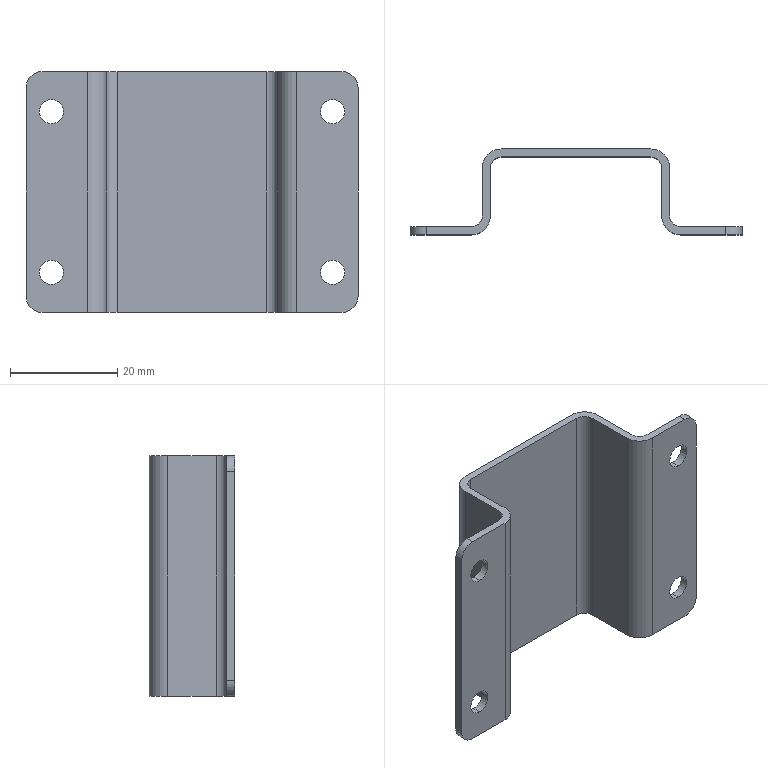Part | SolidWorks | features BaseBody 1 | 1 solid | 34 faces | box 62 x 16 x 45 mm | volume 5717 mm3 | cylinder 20 | plane 14 | commonest cylinder face diameters 4.5 x8 4 x4 6 x4 7 x4
STEP:
#1=CARTESIAN_POINT('',(-26.25,-16.,-17.25));
#2=VERTEX_POINT('',#1);
#3=CARTESIAN_POINT('',(-26.25,-16.,-12.75));
#4=VERTEX_POINT('',#3);
#5=CARTESIAN_POINT('',(-26.25,-16.,-15.));
#6=DIRECTION('',(0.,1.,0.));
#7=DIRECTION('',(0.,0.,1.));
#8=AXIS2_PLACEMENT_3D('',#5,#6,#7);
#9=CIRCLE('',#8,2.25);
#10=EDGE_CURVE('',#2,#4,#9,.T.);
#11=ORIENTED_EDGE('',*,*,#10,.F.);
#12=CARTESIAN_POINT('',(-26.25,-14.5,-17.25));
#13=VERTEX_POINT('',#12);
#14=CARTESIAN_POINT('',(-26.25,-14.5,-17.25));
#15=DIRECTION('',(0.,1.,0.));
#16=VECTOR('',#15,1000.);
#17=LINE('',#14,#16);
#18=EDGE_CURVE('',#2,#13,#17,.T.);
#19=ORIENTED_EDGE('',*,*,#18,.T.);
#20=CARTESIAN_POINT('',(-26.25,-14.5,-12.75));
#21=VERTEX_POINT('',#20);
#22=CARTESIAN_POINT('',(-26.25,-14.5,-15.));
#23=DIRECTION('',(0.,1.,0.));
#24=DIRECTION('',(0.,0.,1.));
#25=AXIS2_PLACEMENT_3D('',#22,#23,#24);
#26=CIRCLE('',#25,2.25);
#27=EDGE_CURVE('',#13,#21,#26,.T.);
#28=ORIENTED_EDGE('',*,*,#27,.T.);
#29=CARTESIAN_POINT('',(-26.25,-14.5,-12.75));
#30=DIRECTION('',(0.,1.,0.));
#31=VECTOR('',#30,1000.);
#32=LINE('',#29,#31);
#33=EDGE_CURVE('',#4,#21,#32,.T.);
#34=ORIENTED_EDGE('',*,*,#33,.F.);
#35=EDGE_LOOP('',(#11,#19,#28,#34));
#36=FACE_OUTER_BOUND('',#35,.T.);
#37=CARTESIAN_POINT('',(-26.25,-14.5,-15.));
#38=DIRECTION('',(0.,1.,0.));
#39=DIRECTION('',(0.,0.,1.));
#40=AXIS2_PLACEMENT_3D('',#37,#38,#39);
#41=CYLINDRICAL_SURFACE('',#40,2.25);
#42=ADVANCED_FACE('',(#36),#41,.F.);
#43=CARTESIAN_POINT('',(-26.25,-16.,12.75));
#44=VERTEX_POINT('',#43);
#45=CARTESIAN_POINT('',(-26.25,-16.,17.25));
#46=VERTEX_POINT('',#45);
#47=CARTESIAN_POINT('',(-26.25,-16.,15.));
#48=DIRECTION('',(0.,1.,0.));
#49=DIRECTION('',(0.,0.,1.));
#50=AXIS2_PLACEMENT_3D('',#47,#48,#49);
#51=CIRCLE('',#50,2.25);
#52=EDGE_CURVE('',#44,#46,#51,.T.);
#53=ORIENTED_EDGE('',*,*,#52,.F.);
#54=CARTESIAN_POINT('',(-26.25,-14.5,12.75));
#55=VERTEX_POINT('',#54);
#56=CARTESIAN_POINT('',(-26.25,-14.5,12.75));
#57=DIRECTION('',(0.,1.,0.));
#58=VECTOR('',#57,1000.);
#59=LINE('',#56,#58);
#60=EDGE_CURVE('',#44,#55,#59,.T.);
#61=ORIENTED_EDGE('',*,*,#60,.T.);
#62=CARTESIAN_POINT('',(-26.25,-14.5,17.25));
#63=VERTEX_POINT('',#62);
#64=CARTESIAN_POINT('',(-26.25,-14.5,15.));
#65=DIRECTION('',(0.,1.,0.));
#66=DIRECTION('',(0.,0.,1.));
#67=AXIS2_PLACEMENT_3D('',#64,#65,#66);
#68=CIRCLE('',#67,2.25);
#69=EDGE_CURVE('',#55,#63,#68,.T.);
#70=ORIENTED_EDGE('',*,*,#69,.T.);
#71=CARTESIAN_POINT('',(-26.25,-14.5,17.25));
#72=DIRECTION('',(0.,1.,0.));
#73=VECTOR('',#72,1000.);
#74=LINE('',#71,#73);
#75=EDGE_CURVE('',#46,#63,#74,.T.);
#76=ORIENTED_EDGE('',*,*,#75,.F.);
#77=EDGE_LOOP('',(#53,#61,#70,#76));
#78=FACE_OUTER_BOUND('',#77,.T.);
#79=CARTESIAN_POINT('',(-26.25,-14.5,15.));
#80=DIRECTION('',(0.,1.,0.));
#81=DIRECTION('',(0.,0.,1.));
#82=AXIS2_PLACEMENT_3D('',#79,#80,#81);
#83=CYLINDRICAL_SURFACE('',#82,2.25);
#84=ADVANCED_FACE('',(#78),#83,.F.);
#85=CARTESIAN_POINT('',(26.25,-16.,12.75));
#86=VERTEX_POINT('',#85);
#87=CARTESIAN_POINT('',(26.25,-16.,17.25));
#88=VERTEX_POINT('',#87);
#89=CARTESIAN_POINT('',(26.25,-16.,15.));
#90=DIRECTION('',(0.,1.,0.));
#91=DIRECTION('',(0.,0.,1.));
#92=AXIS2_PLACEMENT_3D('',#89,#90,#91);
#93=CIRCLE('',#92,2.25);
#94=EDGE_CURVE('',#86,#88,#93,.T.);
#95=ORIENTED_EDGE('',*,*,#94,.F.);
#96=CARTESIAN_POINT('',(26.25,-14.5,12.75));
#97=VERTEX_POINT('',#96);
#98=CARTESIAN_POINT('',(26.25,-14.5,12.75));
#99=DIRECTION('',(0.,1.,0.));
#100=VECTOR('',#99,1000.);
#101=LINE('',#98,#100);
#102=EDGE_CURVE('',#86,#97,#101,.T.);
#103=ORIENTED_EDGE('',*,*,#102,.T.);
#104=CARTESIAN_POINT('',(26.25,-14.5,17.25));
#105=VERTEX_POINT('',#104);
#106=CARTESIAN_POINT('',(26.25,-14.5,15.));
#107=DIRECTION('',(0.,1.,0.));
#108=DIRECTION('',(0.,0.,1.));
#109=AXIS2_PLACEMENT_3D('',#106,#107,#108);
#110=CIRCLE('',#109,2.25);
#111=EDGE_CURVE('',#97,#105,#110,.T.);
#112=ORIENTED_EDGE('',*,*,#111,.T.);
#113=CARTESIAN_POINT('',(26.25,-14.5,17.25));
#114=DIRECTION('',(0.,1.,0.));
#115=VECTOR('',#114,1000.);
#116=LINE('',#113,#115);
#117=EDGE_CURVE('',#88,#105,#116,.T.);
#118=ORIENTED_EDGE('',*,*,#117,.F.);
#119=EDGE_LOOP('',(#95,#103,#112,#118));
#120=FACE_OUTER_BOUND('',#119,.T.);
#121=CARTESIAN_POINT('',(26.25,-14.5,15.));
#122=DIRECTION('',(0.,1.,0.));
#123=DIRECTION('',(0.,0.,1.));
#124=AXIS2_PLACEMENT_3D('',#121,#122,#123);
#125=CYLINDRICAL_SURFACE('',#124,2.25);
#126=ADVANCED_FACE('',(#120),#125,.F.);
#127=CARTESIAN_POINT('',(26.25,-16.,-17.25));
#128=VERTEX_POINT('',#127);
#129=CARTESIAN_POINT('',(26.25,-16.,-12.75));
#130=VERTEX_POINT('',#129);
#131=CARTESIAN_POINT('',(26.25,-16.,-15.));
#132=DIRECTION('',(0.,1.,0.));
#133=DIRECTION('',(0.,0.,1.));
#134=AXIS2_PLACEMENT_3D('',#131,#132,#133);
#135=CIRCLE('',#134,2.25);
#136=EDGE_CURVE('',#128,#130,#135,.T.);
#137=ORIENTED_EDGE('',*,*,#136,.F.);
#138=CARTESIAN_POINT('',(26.25,-14.5,-17.25));
#139=VERTEX_POINT('',#138);
#140=CARTESIAN_POINT('',(26.25,-14.5,-17.25));
#141=DIRECTION('',(0.,1.,0.));
#142=VECTOR('',#141,1000.);
#143=LINE('',#140,#142);
#144=EDGE_CURVE('',#128,#139,#143,.T.);
#145=ORIENTED_EDGE('',*,*,#144,.T.);
#146=CARTESIAN_POINT('',(26.25,-14.5,-12.75));
#147=VERTEX_POINT('',#146);
#148=CARTESIAN_POINT('',(26.25,-14.5,-15.));
#149=DIRECTION('',(0.,1.,0.));
#150=DIRECTION('',(0.,0.,1.));
#151=AXIS2_PLACEMENT_3D('',#148,#149,#150);
#152=CIRCLE('',#151,2.25);
#153=EDGE_CURVE('',#139,#147,#152,.T.);
#154=ORIENTED_EDGE('',*,*,#153,.T.);
#155=CARTESIAN_POINT('',(26.25,-14.5,-12.75));
#156=DIRECTION('',(0.,1.,0.));
#157=VECTOR('',#156,1000.);
#158=LINE('',#155,#157);
#159=EDGE_CURVE('',#130,#147,#158,.T.);
#160=ORIENTED_EDGE('',*,*,#159,.F.);
#161=EDGE_LOOP('',(#137,#145,#154,#160));
#162=FACE_OUTER_BOUND('',#161,.T.);
#163=CARTESIAN_POINT('',(26.25,-14.5,-15.));
#164=DIRECTION('',(0.,1.,0.));
#165=DIRECTION('',(0.,0.,1.));
#166=AXIS2_PLACEMENT_3D('',#163,#164,#165);
#167=CYLINDRICAL_SURFACE('',#166,2.25);
#168=ADVANCED_FACE('',(#162),#167,.F.);
#169=CARTESIAN_POINT('',(28.,-16.,-22.5));
#170=VERTEX_POINT('',#169);
#171=CARTESIAN_POINT('',(31.,-16.,-19.5));
#172=VERTEX_POINT('',#171);
#173=CARTESIAN_POINT('',(28.,-16.,-19.5));
#174=DIRECTION('',(0.,-1.,0.));
#175=DIRECTION('',(0.,0.,1.));
#176=AXIS2_PLACEMENT_3D('',#173,#174,#175);
#177=CIRCLE('',#176,3.);
#178=EDGE_CURVE('',#170,#172,#177,.T.);
#179=ORIENTED_EDGE('',*,*,#178,.F.);
#180=CARTESIAN_POINT('',(28.,-14.5,-22.5));
#181=VERTEX_POINT('',#180);
#182=CARTESIAN_POINT('',(28.,-16.,-22.5));
#183=DIRECTION('',(0.,-1.,0.));
#184=VECTOR('',#183,1000.);
#185=LINE('',#182,#184);
#186=EDGE_CURVE('',#181,#170,#185,.T.);
#187=ORIENTED_EDGE('',*,*,#186,.F.);
#188=CARTESIAN_POINT('',(31.,-14.5,-19.5));
#189=VERTEX_POINT('',#188);
#190=CARTESIAN_POINT('',(28.,-14.5,-19.5));
#191=DIRECTION('',(0.,1.,0.));
#192=DIRECTION('',(0.,0.,1.));
#193=AXIS2_PLACEMENT_3D('',#190,#191,#192);
#194=CIRCLE('',#193,3.);
#195=EDGE_CURVE('',#189,#181,#194,.T.);
#196=ORIENTED_EDGE('',*,*,#195,.F.);
#197=CARTESIAN_POINT('',(31.,-16.,-19.5));
#198=DIRECTION('',(0.,1.,0.));
#199=VECTOR('',#198,1000.);
#200=LINE('',#197,#199);
#201=EDGE_CURVE('',#172,#189,#200,.T.);
#202=ORIENTED_EDGE('',*,*,#201,.F.);
#203=EDGE_LOOP('',(#179,#187,#196,#202));
#204=FACE_OUTER_BOUND('',#203,.T.);
#205=CARTESIAN_POINT('',(28.,-16.,-19.5));
#206=DIRECTION('',(0.,1.,0.));
#207=DIRECTION('',(-1.,0.,0.));
#208=AXIS2_PLACEMENT_3D('',#205,#206,#207);
#209=CYLINDRICAL_SURFACE('',#208,3.);
#210=ADVANCED_FACE('',(#204),#209,.T.);
#211=CARTESIAN_POINT('',(31.,-16.,19.5));
#212=VERTEX_POINT('',#211);
#213=CARTESIAN_POINT('',(28.,-16.,22.5));
#214=VERTEX_POINT('',#213);
#215=CARTESIAN_POINT('',(28.,-16.,19.5));
#216=DIRECTION('',(0.,-1.,0.));
#217=DIRECTION('',(0.,0.,1.));
#218=AXIS2_PLACEMENT_3D('',#215,#216,#217);
#219=CIRCLE('',#218,3.);
#220=EDGE_CURVE('',#212,#214,#219,.T.);
#221=ORIENTED_EDGE('',*,*,#220,.F.);
#222=CARTESIAN_POINT('',(31.,-14.5,19.5));
#223=VERTEX_POINT('',#222);
#224=CARTESIAN_POINT('',(31.,-16.,19.5));
#225=DIRECTION('',(0.,-1.,0.));
#226=VECTOR('',#225,1000.);
#227=LINE('',#224,#226);
#228=EDGE_CURVE('',#223,#212,#227,.T.);
#229=ORIENTED_EDGE('',*,*,#228,.F.);
#230=CARTESIAN_POINT('',(28.,-14.5,22.5));
#231=VERTEX_POINT('',#230);
#232=CARTESIAN_POINT('',(28.,-14.5,19.5));
#233=DIRECTION('',(0.,1.,0.));
#234=DIRECTION('',(0.,0.,1.));
#235=AXIS2_PLACEMENT_3D('',#232,#233,#234);
#236=CIRCLE('',#235,3.);
#237=EDGE_CURVE('',#231,#223,#236,.T.);
#238=ORIENTED_EDGE('',*,*,#237,.F.);
#239=CARTESIAN_POINT('',(28.,-16.,22.5));
#240=DIRECTION('',(0.,1.,0.));
#241=VECTOR('',#240,1000.);
#242=LINE('',#239,#241);
#243=EDGE_CURVE('',#214,#231,#242,.T.);
#244=ORIENTED_EDGE('',*,*,#243,.F.);
#245=EDGE_LOOP('',(#221,#229,#238,#244));
#246=FACE_OUTER_BOUND('',#245,.T.);
#247=CARTESIAN_POINT('',(28.,-16.,19.5));
#248=DIRECTION('',(0.,1.,0.));
#249=DIRECTION('',(-1.,0.,0.));
#250=AXIS2_PLACEMENT_3D('',#247,#248,#249);
#251=CYLINDRICAL_SURFACE('',#250,3.);
#252=ADVANCED_FACE('',(#246),#251,.T.);
#253=CARTESIAN_POINT('',(-28.,-16.,22.5));
#254=VERTEX_POINT('',#253);
#255=CARTESIAN_POINT('',(-31.,-16.,19.5));
#256=VERTEX_POINT('',#255);
#257=CARTESIAN_POINT('',(-28.,-16.,19.5));
#258=DIRECTION('',(0.,-1.,0.));
#259=DIRECTION('',(0.,0.,1.));
#260=AXIS2_PLACEMENT_3D('',#257,#258,#259);
#261=CIRCLE('',#260,3.);
#262=EDGE_CURVE('',#254,#256,#261,.T.);
#263=ORIENTED_EDGE('',*,*,#262,.F.);
#264=CARTESIAN_POINT('',(-28.,-14.5,22.5));
#265=VERTEX_POINT('',#264);
#266=CARTESIAN_POINT('',(-28.,-16.,22.5));
#267=DIRECTION('',(0.,-1.,0.));
#268=VECTOR('',#267,1000.);
#269=LINE('',#266,#268);
#270=EDGE_CURVE('',#265,#254,#269,.T.);
#271=ORIENTED_EDGE('',*,*,#270,.F.);
#272=CARTESIAN_POINT('',(-31.,-14.5,19.5));
#273=VERTEX_POINT('',#272);
#274=CARTESIAN_POINT('',(-28.,-14.5,19.5));
#275=DIRECTION('',(0.,1.,0.));
#276=DIRECTION('',(0.,0.,1.));
#277=AXIS2_PLACEMENT_3D('',#274,#275,#276);
#278=CIRCLE('',#277,3.);
#279=EDGE_CURVE('',#273,#265,#278,.T.);
#280=ORIENTED_EDGE('',*,*,#279,.F.);
#281=CARTESIAN_POINT('',(-31.,-16.,19.5));
#282=DIRECTION('',(0.,1.,0.));
#283=VECTOR('',#282,1000.);
#284=LINE('',#281,#283);
#285=EDGE_CURVE('',#256,#273,#284,.T.);
#286=ORIENTED_EDGE('',*,*,#285,.F.);
#287=EDGE_LOOP('',(#263,#271,#280,#286));
#288=FACE_OUTER_BOUND('',#287,.T.);
#289=CARTESIAN_POINT('',(-28.,-16.,19.5));
#290=DIRECTION('',(0.,1.,0.));
#291=DIRECTION('',(-1.,0.,0.));
#292=AXIS2_PLACEMENT_3D('',#289,#290,#291);
#293=CYLINDRICAL_SURFACE('',#292,3.);
#294=ADVANCED_FACE('',(#288),#293,.T.);
#295=CARTESIAN_POINT('',(-31.,-16.,-19.5));
#296=VERTEX_POINT('',#295);
#297=CARTESIAN_POINT('',(-28.,-16.,-22.5));
#298=VERTEX_POINT('',#297);
#299=CARTESIAN_POINT('',(-28.,-16.,-19.5));
#300=DIRECTION('',(0.,-1.,0.));
#301=DIRECTION('',(0.,0.,1.));
#302=AXIS2_PLACEMENT_3D('',#299,#300,#301);
#303=CIRCLE('',#302,3.);
#304=EDGE_CURVE('',#296,#298,#303,.T.);
#305=ORIENTED_EDGE('',*,*,#304,.F.);
#306=CARTESIAN_POINT('',(-31.,-14.5,-19.5));
#307=VERTEX_POINT('',#306);
#308=CARTESIAN_POINT('',(-31.,-16.,-19.5));
#309=DIRECTION('',(0.,-1.,0.));
#310=VECTOR('',#309,1000.);
#311=LINE('',#308,#310);
#312=EDGE_CURVE('',#307,#296,#311,.T.);
#313=ORIENTED_EDGE('',*,*,#312,.F.);
#314=CARTESIAN_POINT('',(-28.,-14.5,-22.5));
#315=VERTEX_POINT('',#314);
#316=CARTESIAN_POINT('',(-28.,-14.5,-19.5));
#317=DIRECTION('',(0.,1.,0.));
#318=DIRECTION('',(0.,0.,1.));
#319=AXIS2_PLACEMENT_3D('',#316,#317,#318);
#320=CIRCLE('',#319,3.);
#321=EDGE_CURVE('',#315,#307,#320,.T.);
#322=ORIENTED_EDGE('',*,*,#321,.F.);
#323=CARTESIAN_POINT('',(-28.,-16.,-22.5));
#324=DIRECTION('',(0.,1.,0.));
#325=VECTOR('',#324,1000.);
#326=LINE('',#323,#325);
#327=EDGE_CURVE('',#298,#315,#326,.T.);
#328=ORIENTED_EDGE('',*,*,#327,.F.);
#329=EDGE_LOOP('',(#305,#313,#322,#328));
#330=FACE_OUTER_BOUND('',#329,.T.);
#331=CARTESIAN_POINT('',(-28.,-16.,-19.5));
#332=DIRECTION('',(0.,1.,0.));
#333=DIRECTION('',(-1.,0.,0.));
#334=AXIS2_PLACEMENT_3D('',#331,#332,#333);
#335=CYLINDRICAL_SURFACE('',#334,3.);
#336=ADVANCED_FACE('',(#330),#335,.T.);
#337=CARTESIAN_POINT('',(31.,-14.5,22.5));
#338=DIRECTION('',(0.,0.,1.));
#339=VECTOR('',#338,1000.);
#340=LINE('',#337,#339);
#341=EDGE_CURVE('',#189,#223,#340,.T.);
#342=ORIENTED_EDGE('',*,*,#341,.T.);
#343=ORIENTED_EDGE('',*,*,#228,.T.);
#344=CARTESIAN_POINT('',(31.,-16.,0.));
#345=DIRECTION('',(0.,0.,1.));
#346=VECTOR('',#345,1000.);
#347=LINE('',#344,#346);
#348=EDGE_CURVE('',#172,#212,#347,.T.);
#349=ORIENTED_EDGE('',*,*,#348,.F.);
#350=ORIENTED_EDGE('',*,*,#201,.T.);
#351=EDGE_LOOP('',(#342,#343,#349,#350));
#352=FACE_OUTER_BOUND('',#351,.T.);
#353=CARTESIAN_POINT('',(31.,-16.,22.5));
#354=DIRECTION('',(-1.,0.,0.));
#355=DIRECTION('',(0.,1.,0.));
#356=AXIS2_PLACEMENT_3D('',#353,#354,#355);
#357=PLANE('',#356);
#358=ADVANCED_FACE('',(#352),#357,.F.);
#359=CARTESIAN_POINT('',(26.25,-14.5,-15.));
#360=DIRECTION('',(0.,1.,0.));
#361=DIRECTION('',(0.,0.,1.));
#362=AXIS2_PLACEMENT_3D('',#359,#360,#361);
#363=CIRCLE('',#362,2.25);
#364=EDGE_CURVE('',#147,#139,#363,.T.);
#365=ORIENTED_EDGE('',*,*,#364,.F.);
#366=ORIENTED_EDGE('',*,*,#153,.F.);
#367=EDGE_LOOP('',(#365,#366));
#368=FACE_BOUND('',#367,.T.);
#369=CARTESIAN_POINT('',(26.25,-14.5,15.));
#370=DIRECTION('',(0.,1.,0.));
#371=DIRECTION('',(0.,0.,1.));
#372=AXIS2_PLACEMENT_3D('',#369,#370,#371);
#373=CIRCLE('',#372,2.25);
#374=EDGE_CURVE('',#105,#97,#373,.T.);
#375=ORIENTED_EDGE('',*,*,#374,.F.);
#376=ORIENTED_EDGE('',*,*,#111,.F.);
#377=EDGE_LOOP('',(#375,#376));
#378=FACE_BOUND('',#377,.T.);
#379=CARTESIAN_POINT('',(19.5,-14.5,22.5));
#380=VERTEX_POINT('',#379);
#381=CARTESIAN_POINT('',(17.5,-14.5,22.5));
#382=DIRECTION('',(-1.,0.,0.));
#383=VECTOR('',#382,1000.);
#384=LINE('',#381,#383);
#385=EDGE_CURVE('',#231,#380,#384,.T.);
#386=ORIENTED_EDGE('',*,*,#385,.F.);
#387=ORIENTED_EDGE('',*,*,#237,.T.);
#388=ORIENTED_EDGE('',*,*,#341,.F.);
#389=ORIENTED_EDGE('',*,*,#195,.T.);
#390=CARTESIAN_POINT('',(19.5,-14.5,-22.5));
#391=VERTEX_POINT('',#390);
#392=CARTESIAN_POINT('',(31.,-14.5,-22.5));
#393=DIRECTION('',(1.,0.,0.));
#394=VECTOR('',#393,1000.);
#395=LINE('',#392,#394);
#396=EDGE_CURVE('',#391,#181,#395,.T.);
#397=ORIENTED_EDGE('',*,*,#396,.F.);
#398=CARTESIAN_POINT('',(19.5,-14.5,22.5));
#399=DIRECTION('',(0.,0.,-1.));
#400=VECTOR('',#399,1000.);
#401=LINE('',#398,#400);
#402=EDGE_CURVE('',#380,#391,#401,.T.);
#403=ORIENTED_EDGE('',*,*,#402,.F.);
#404=EDGE_LOOP('',(#386,#387,#388,#389,#397,#403));
#405=FACE_OUTER_BOUND('',#404,.T.);
#406=CARTESIAN_POINT('',(0.,-14.5,0.));
#407=DIRECTION('',(0.,1.,0.));
#408=DIRECTION('',(1.,0.,0.));
#409=AXIS2_PLACEMENT_3D('',#406,#407,#408);
#410=PLANE('',#409);
#411=ADVANCED_FACE('',(#368,#378,#405),#410,.T.);
#412=CARTESIAN_POINT('',(26.25,-16.,-15.));
#413=DIRECTION('',(0.,1.,0.));
#414=DIRECTION('',(0.,0.,1.));
#415=AXIS2_PLACEMENT_3D('',#412,#413,#414);
#416=CIRCLE('',#415,2.25);
#417=EDGE_CURVE('',#130,#128,#416,.T.);
#418=ORIENTED_EDGE('',*,*,#417,.T.);
#419=ORIENTED_EDGE('',*,*,#136,.T.);
#420=EDGE_LOOP('',(#418,#419));
#421=FACE_BOUND('',#420,.T.);
#422=CARTESIAN_POINT('',(26.25,-16.,15.));
#423=DIRECTION('',(0.,1.,0.));
#424=DIRECTION('',(0.,0.,1.));
#425=AXIS2_PLACEMENT_3D('',#422,#423,#424);
#426=CIRCLE('',#425,2.25);
#427=EDGE_CURVE('',#88,#86,#426,.T.);
#428=ORIENTED_EDGE('',*,*,#427,.T.);
#429=ORIENTED_EDGE('',*,*,#94,.T.);
#430=EDGE_LOOP('',(#428,#429));
#431=FACE_BOUND('',#430,.T.);
#432=ORIENTED_EDGE('',*,*,#348,.T.);
#433=ORIENTED_EDGE('',*,*,#220,.T.);
#434=CARTESIAN_POINT('',(19.5,-16.,22.5));
#435=VERTEX_POINT('',#434);
#436=CARTESIAN_POINT('',(0.,-16.,22.5));
#437=DIRECTION('',(-1.,0.,0.));
#438=VECTOR('',#437,1000.);
#439=LINE('',#436,#438);
#440=EDGE_CURVE('',#214,#435,#439,.T.);
#441=ORIENTED_EDGE('',*,*,#440,.T.);
#442=CARTESIAN_POINT('',(19.5,-16.,-22.5));
#443=VERTEX_POINT('',#442);
#444=CARTESIAN_POINT('',(19.5,-16.,22.5));
#445=DIRECTION('',(0.,0.,1.));
#446=VECTOR('',#445,1000.);
#447=LINE('',#444,#446);
#448=EDGE_CURVE('',#443,#435,#447,.T.);
#449=ORIENTED_EDGE('',*,*,#448,.F.);
#450=CARTESIAN_POINT('',(0.,-16.,-22.5));
#451=DIRECTION('',(1.,0.,0.));
#452=VECTOR('',#451,1000.);
#453=LINE('',#450,#452);
#454=EDGE_CURVE('',#443,#170,#453,.T.);
#455=ORIENTED_EDGE('',*,*,#454,.T.);
#456=ORIENTED_EDGE('',*,*,#178,.T.);
#457=EDGE_LOOP('',(#432,#433,#441,#449,#455,#456));
#458=FACE_OUTER_BOUND('',#457,.T.);
#459=CARTESIAN_POINT('',(0.,-16.,0.));
#460=DIRECTION('',(0.,1.,0.));
#461=DIRECTION('',(1.,0.,0.));
#462=AXIS2_PLACEMENT_3D('',#459,#460,#461);
#463=PLANE('',#462);
#464=ADVANCED_FACE('',(#421,#431,#458),#463,.F.);
#465=CARTESIAN_POINT('',(17.5,-12.5,-22.5));
#466=VERTEX_POINT('',#465);
#467=CARTESIAN_POINT('',(17.5,-12.5,22.5));
#468=VERTEX_POINT('',#467);
#469=CARTESIAN_POINT('',(17.5,-12.5,-22.5));
#470=DIRECTION('',(0.,0.,1.));
#471=VECTOR('',#470,1000.);
#472=LINE('',#469,#471);
#473=EDGE_CURVE('',#466,#468,#472,.T.);
#474=ORIENTED_EDGE('',*,*,#473,.T.);
#475=CARTESIAN_POINT('',(19.5,-12.5,22.5));
#476=DIRECTION('',(0.,0.,1.));
#477=DIRECTION('',(-1.,0.,0.));
#478=AXIS2_PLACEMENT_3D('',#475,#476,#477);
#479=CIRCLE('',#478,2.);
#480=EDGE_CURVE('',#468,#380,#479,.T.);
#481=ORIENTED_EDGE('',*,*,#480,.T.);
#482=ORIENTED_EDGE('',*,*,#402,.T.);
#483=CARTESIAN_POINT('',(19.5,-12.5,-22.5));
#484=DIRECTION('',(0.,0.,-1.));
#485=DIRECTION('',(-1.,0.,0.));
#486=AXIS2_PLACEMENT_3D('',#483,#484,#485);
#487=CIRCLE('',#486,2.);
#488=EDGE_CURVE('',#391,#466,#487,.T.);
#489=ORIENTED_EDGE('',*,*,#488,.T.);
#490=EDGE_LOOP('',(#474,#481,#482,#489));
#491=FACE_OUTER_BOUND('',#490,.T.);
#492=CARTESIAN_POINT('',(19.5,-12.5,-22.5));
#493=DIRECTION('',(0.,0.,-1.));
#494=DIRECTION('',(0.,-1.,0.));
#495=AXIS2_PLACEMENT_3D('',#492,#493,#494);
#496=CYLINDRICAL_SURFACE('',#495,2.);
#497=ADVANCED_FACE('',(#491),#496,.F.);
#498=CARTESIAN_POINT('',(16.,-12.5,-22.5));
#499=VERTEX_POINT('',#498);
#500=CARTESIAN_POINT('',(16.,-12.5,22.5));
#501=VERTEX_POINT('',#500);
#502=CARTESIAN_POINT('',(16.,-12.5,-22.5));
#503=DIRECTION('',(0.,0.,1.));
#504=VECTOR('',#503,1000.);
#505=LINE('',#502,#504);
#506=EDGE_CURVE('',#499,#501,#505,.T.);
#507=ORIENTED_EDGE('',*,*,#506,.F.);
#508=CARTESIAN_POINT('',(19.5,-12.5,-22.5));
#509=DIRECTION('',(0.,0.,-1.));
#510=DIRECTION('',(-1.,0.,0.));
#511=AXIS2_PLACEMENT_3D('',#508,#509,#510);
#512=CIRCLE('',#511,3.5);
#513=EDGE_CURVE('',#443,#499,#512,.T.);
#514=ORIENTED_EDGE('',*,*,#513,.F.);
#515=ORIENTED_EDGE('',*,*,#448,.T.);
#516=CARTESIAN_POINT('',(19.5,-12.5,22.5));
#517=DIRECTION('',(0.,0.,1.));
#518=DIRECTION('',(-1.,0.,0.));
#519=AXIS2_PLACEMENT_3D('',#516,#517,#518);
#520=CIRCLE('',#519,3.5);
#521=EDGE_CURVE('',#501,#435,#520,.T.);
#522=ORIENTED_EDGE('',*,*,#521,.F.);
#523=EDGE_LOOP('',(#507,#514,#515,#522));
#524=FACE_OUTER_BOUND('',#523,.T.);
#525=CARTESIAN_POINT('',(19.5,-12.5,-22.5));
#526=DIRECTION('',(0.,0.,-1.));
#527=DIRECTION('',(0.,-1.,0.));
#528=AXIS2_PLACEMENT_3D('',#525,#526,#527);
#529=CYLINDRICAL_SURFACE('',#528,3.5);
#530=ADVANCED_FACE('',(#524),#529,.T.);
#531=CARTESIAN_POINT('',(-31.,-14.5,-22.5));
#532=DIRECTION('',(0.,0.,-1.));
#533=VECTOR('',#532,1000.);
#534=LINE('',#531,#533);
#535=EDGE_CURVE('',#273,#307,#534,.T.);
#536=ORIENTED_EDGE('',*,*,#535,.T.);
#537=ORIENTED_EDGE('',*,*,#312,.T.);
#538=CARTESIAN_POINT('',(-31.,-16.,0.));
#539=DIRECTION('',(0.,0.,-1.));
#540=VECTOR('',#539,1000.);
#541=LINE('',#538,#540);
#542=EDGE_CURVE('',#256,#296,#541,.T.);
#543=ORIENTED_EDGE('',*,*,#542,.F.);
#544=ORIENTED_EDGE('',*,*,#285,.T.);
#545=EDGE_LOOP('',(#536,#537,#543,#544));
#546=FACE_OUTER_BOUND('',#545,.T.);
#547=CARTESIAN_POINT('',(-31.,-16.,-22.5));
#548=DIRECTION('',(1.,0.,0.));
#549=DIRECTION('',(0.,0.,-1.));
#550=AXIS2_PLACEMENT_3D('',#547,#548,#549);
#551=PLANE('',#550);
#552=ADVANCED_FACE('',(#546),#551,.F.);
#553=CARTESIAN_POINT('',(-26.25,-14.5,15.));
#554=DIRECTION('',(0.,1.,0.));
#555=DIRECTION('',(0.,0.,1.));
#556=AXIS2_PLACEMENT_3D('',#553,#554,#555);
#557=CIRCLE('',#556,2.25);
#558=EDGE_CURVE('',#63,#55,#557,.T.);
#559=ORIENTED_EDGE('',*,*,#558,.F.);
#560=ORIENTED_EDGE('',*,*,#69,.F.);
#561=EDGE_LOOP('',(#559,#560));
#562=FACE_BOUND('',#561,.T.);
#563=CARTESIAN_POINT('',(-26.25,-14.5,-15.));
#564=DIRECTION('',(0.,1.,0.));
#565=DIRECTION('',(0.,0.,1.));
#566=AXIS2_PLACEMENT_3D('',#563,#564,#565);
#567=CIRCLE('',#566,2.25);
#568=EDGE_CURVE('',#21,#13,#567,.T.);
#569=ORIENTED_EDGE('',*,*,#568,.F.);
#570=ORIENTED_EDGE('',*,*,#27,.F.);
#571=EDGE_LOOP('',(#569,#570));
#572=FACE_BOUND('',#571,.T.);
#573=CARTESIAN_POINT('',(-19.5,-14.5,-22.5));
#574=VERTEX_POINT('',#573);
#575=CARTESIAN_POINT('',(-17.5,-14.5,-22.5));
#576=DIRECTION('',(1.,0.,0.));
#577=VECTOR('',#576,1000.);
#578=LINE('',#575,#577);
#579=EDGE_CURVE('',#315,#574,#578,.T.);
#580=ORIENTED_EDGE('',*,*,#579,.F.);
#581=ORIENTED_EDGE('',*,*,#321,.T.);
#582=ORIENTED_EDGE('',*,*,#535,.F.);
#583=ORIENTED_EDGE('',*,*,#279,.T.);
#584=CARTESIAN_POINT('',(-19.5,-14.5,22.5));
#585=VERTEX_POINT('',#584);
#586=CARTESIAN_POINT('',(-31.,-14.5,22.5));
#587=DIRECTION('',(-1.,0.,0.));
#588=VECTOR('',#587,1000.);
#589=LINE('',#586,#588);
#590=EDGE_CURVE('',#585,#265,#589,.T.);
#591=ORIENTED_EDGE('',*,*,#590,.F.);
#592=CARTESIAN_POINT('',(-19.5,-14.5,-22.5));
#593=DIRECTION('',(0.,0.,1.));
#594=VECTOR('',#593,1000.);
#595=LINE('',#592,#594);
#596=EDGE_CURVE('',#574,#585,#595,.T.);
#597=ORIENTED_EDGE('',*,*,#596,.F.);
#598=EDGE_LOOP('',(#580,#581,#582,#583,#591,#597));
#599=FACE_OUTER_BOUND('',#598,.T.);
#600=CARTESIAN_POINT('',(0.,-14.5,0.));
#601=DIRECTION('',(0.,1.,0.));
#602=DIRECTION('',(1.,0.,0.));
#603=AXIS2_PLACEMENT_3D('',#600,#601,#602);
#604=PLANE('',#603);
#605=ADVANCED_FACE('',(#562,#572,#599),#604,.T.);
#606=CARTESIAN_POINT('',(-26.25,-16.,15.));
#607=DIRECTION('',(0.,1.,0.));
#608=DIRECTION('',(0.,0.,1.));
#609=AXIS2_PLACEMENT_3D('',#606,#607,#608);
#610=CIRCLE('',#609,2.25);
#611=EDGE_CURVE('',#46,#44,#610,.T.);
#612=ORIENTED_EDGE('',*,*,#611,.T.);
#613=ORIENTED_EDGE('',*,*,#52,.T.);
#614=EDGE_LOOP('',(#612,#613));
#615=FACE_BOUND('',#614,.T.);
#616=CARTESIAN_POINT('',(-26.25,-16.,-15.));
#617=DIRECTION('',(0.,1.,0.));
#618=DIRECTION('',(0.,0.,1.));
#619=AXIS2_PLACEMENT_3D('',#616,#617,#618);
#620=CIRCLE('',#619,2.25);
#621=EDGE_CURVE('',#4,#2,#620,.T.);
#622=ORIENTED_EDGE('',*,*,#621,.T.);
#623=ORIENTED_EDGE('',*,*,#10,.T.);
#624=EDGE_LOOP('',(#622,#623));
#625=FACE_BOUND('',#624,.T.);
#626=ORIENTED_EDGE('',*,*,#542,.T.);
#627=ORIENTED_EDGE('',*,*,#304,.T.);
#628=CARTESIAN_POINT('',(-19.5,-16.,-22.5));
#629=VERTEX_POINT('',#628);
#630=CARTESIAN_POINT('',(0.,-16.,-22.5));
#631=DIRECTION('',(1.,0.,0.));
#632=VECTOR('',#631,1000.);
#633=LINE('',#630,#632);
#634=EDGE_CURVE('',#298,#629,#633,.T.);
#635=ORIENTED_EDGE('',*,*,#634,.T.);
#636=CARTESIAN_POINT('',(-19.5,-16.,22.5));
#637=VERTEX_POINT('',#636);
#638=CARTESIAN_POINT('',(-19.5,-16.,-22.5));
#639=DIRECTION('',(0.,0.,-1.));
#640=VECTOR('',#639,1000.);
#641=LINE('',#638,#640);
#642=EDGE_CURVE('',#637,#629,#641,.T.);
#643=ORIENTED_EDGE('',*,*,#642,.F.);
#644=CARTESIAN_POINT('',(0.,-16.,22.5));
#645=DIRECTION('',(-1.,0.,0.));
#646=VECTOR('',#645,1000.);
#647=LINE('',#644,#646);
#648=EDGE_CURVE('',#637,#254,#647,.T.);
#649=ORIENTED_EDGE('',*,*,#648,.T.);
#650=ORIENTED_EDGE('',*,*,#262,.T.);
#651=EDGE_LOOP('',(#626,#627,#635,#643,#649,#650));
#652=FACE_OUTER_BOUND('',#651,.T.);
#653=CARTESIAN_POINT('',(0.,-16.,0.));
#654=DIRECTION('',(0.,1.,0.));
#655=DIRECTION('',(1.,0.,0.));
#656=AXIS2_PLACEMENT_3D('',#653,#654,#655);
#657=PLANE('',#656);
#658=ADVANCED_FACE('',(#615,#625,#652),#657,.F.);
#659=CARTESIAN_POINT('',(-17.5,-12.5,22.5));
#660=VERTEX_POINT('',#659);
#661=CARTESIAN_POINT('',(-17.5,-12.5,-22.5));
#662=VERTEX_POINT('',#661);
#663=CARTESIAN_POINT('',(-17.5,-12.5,22.5));
#664=DIRECTION('',(0.,0.,-1.));
#665=VECTOR('',#664,1000.);
#666=LINE('',#663,#665);
#667=EDGE_CURVE('',#660,#662,#666,.T.);
#668=ORIENTED_EDGE('',*,*,#667,.T.);
#669=CARTESIAN_POINT('',(-19.5,-12.5,-22.5));
#670=DIRECTION('',(0.,0.,-1.));
#671=DIRECTION('',(1.,0.,0.));
#672=AXIS2_PLACEMENT_3D('',#669,#670,#671);
#673=CIRCLE('',#672,2.);
#674=EDGE_CURVE('',#662,#574,#673,.T.);
#675=ORIENTED_EDGE('',*,*,#674,.T.);
#676=ORIENTED_EDGE('',*,*,#596,.T.);
#677=CARTESIAN_POINT('',(-19.5,-12.5,22.5));
#678=DIRECTION('',(0.,0.,1.));
#679=DIRECTION('',(1.,0.,0.));
#680=AXIS2_PLACEMENT_3D('',#677,#678,#679);
#681=CIRCLE('',#680,2.);
#682=EDGE_CURVE('',#585,#660,#681,.T.);
#683=ORIENTED_EDGE('',*,*,#682,.T.);
#684=EDGE_LOOP('',(#668,#675,#676,#683));
#685=FACE_OUTER_BOUND('',#684,.T.);
#686=CARTESIAN_POINT('',(-19.5,-12.5,22.5));
#687=DIRECTION('',(0.,0.,1.));
#688=DIRECTION('',(0.,-1.,0.));
#689=AXIS2_PLACEMENT_3D('',#686,#687,#688);
#690=CYLINDRICAL_SURFACE('',#689,2.);
#691=ADVANCED_FACE('',(#685),#690,.F.);
#692=CARTESIAN_POINT('',(-16.,-12.5,22.5));
#693=VERTEX_POINT('',#692);
#694=CARTESIAN_POINT('',(-16.,-12.5,-22.5));
#695=VERTEX_POINT('',#694);
#696=CARTESIAN_POINT('',(-16.,-12.5,22.5));
#697=DIRECTION('',(0.,0.,-1.));
#698=VECTOR('',#697,1000.);
#699=LINE('',#696,#698);
#700=EDGE_CURVE('',#693,#695,#699,.T.);
#701=ORIENTED_EDGE('',*,*,#700,.F.);
#702=CARTESIAN_POINT('',(-19.5,-12.5,22.5));
#703=DIRECTION('',(0.,0.,1.));
#704=DIRECTION('',(1.,0.,0.));
#705=AXIS2_PLACEMENT_3D('',#702,#703,#704);
#706=CIRCLE('',#705,3.5);
#707=EDGE_CURVE('',#637,#693,#706,.T.);
#708=ORIENTED_EDGE('',*,*,#707,.F.);
#709=ORIENTED_EDGE('',*,*,#642,.T.);
#710=CARTESIAN_POINT('',(-19.5,-12.5,-22.5));
#711=DIRECTION('',(0.,0.,-1.));
#712=DIRECTION('',(1.,0.,0.));
#713=AXIS2_PLACEMENT_3D('',#710,#711,#712);
#714=CIRCLE('',#713,3.5);
#715=EDGE_CURVE('',#695,#629,#714,.T.);
#716=ORIENTED_EDGE('',*,*,#715,.F.);
#717=EDGE_LOOP('',(#701,#708,#709,#716));
#718=FACE_OUTER_BOUND('',#717,.T.);
#719=CARTESIAN_POINT('',(-19.5,-12.5,22.5));
#720=DIRECTION('',(0.,0.,1.));
#721=DIRECTION('',(0.,-1.,0.));
#722=AXIS2_PLACEMENT_3D('',#719,#720,#721);
#723=CYLINDRICAL_SURFACE('',#722,3.5);
#724=ADVANCED_FACE('',(#718),#723,.T.);
#725=CARTESIAN_POINT('',(-14.,-1.5,-22.5));
#726=VERTEX_POINT('',#725);
#727=CARTESIAN_POINT('',(-14.,-1.5,22.5));
#728=VERTEX_POINT('',#727);
#729=CARTESIAN_POINT('',(-14.,-1.5,-22.5));
#730=DIRECTION('',(0.,0.,1.));
#731=VECTOR('',#730,1000.);
#732=LINE('',#729,#731);
#733=EDGE_CURVE('',#726,#728,#732,.T.);
#734=ORIENTED_EDGE('',*,*,#733,.T.);
#735=CARTESIAN_POINT('',(-16.,-3.5,22.5));
#736=VERTEX_POINT('',#735);
#737=CARTESIAN_POINT('',(-14.,-3.5,22.5));
#738=DIRECTION('',(0.,0.,1.));
#739=DIRECTION('',(-1.,0.,0.));
#740=AXIS2_PLACEMENT_3D('',#737,#738,#739);
#741=CIRCLE('',#740,2.);
#742=EDGE_CURVE('',#728,#736,#741,.T.);
#743=ORIENTED_EDGE('',*,*,#742,.T.);
#744=CARTESIAN_POINT('',(-16.,-3.5,-22.5));
#745=VERTEX_POINT('',#744);
#746=CARTESIAN_POINT('',(-16.,-3.5,22.5));
#747=DIRECTION('',(0.,0.,-1.));
#748=VECTOR('',#747,1000.);
#749=LINE('',#746,#748);
#750=EDGE_CURVE('',#736,#745,#749,.T.);
#751=ORIENTED_EDGE('',*,*,#750,.T.);
#752=CARTESIAN_POINT('',(-14.,-3.5,-22.5));
#753=DIRECTION('',(0.,0.,-1.));
#754=DIRECTION('',(-1.,0.,0.));
#755=AXIS2_PLACEMENT_3D('',#752,#753,#754);
#756=CIRCLE('',#755,2.);
#757=EDGE_CURVE('',#745,#726,#756,.T.);
#758=ORIENTED_EDGE('',*,*,#757,.T.);
#759=EDGE_LOOP('',(#734,#743,#751,#758));
#760=FACE_OUTER_BOUND('',#759,.T.);
#761=CARTESIAN_POINT('',(-14.,-3.5,-22.5));
#762=DIRECTION('',(0.,0.,-1.));
#763=DIRECTION('',(-1.,0.,0.));
#764=AXIS2_PLACEMENT_3D('',#761,#762,#763);
#765=CYLINDRICAL_SURFACE('',#764,2.);
#766=ADVANCED_FACE('',(#760),#765,.F.);
#767=CARTESIAN_POINT('',(-14.,0.,-22.5));
#768=VERTEX_POINT('',#767);
#769=CARTESIAN_POINT('',(-14.,0.,22.5));
#770=VERTEX_POINT('',#769);
#771=CARTESIAN_POINT('',(-14.,0.,-22.5));
#772=DIRECTION('',(0.,0.,1.));
#773=VECTOR('',#772,1000.);
#774=LINE('',#771,#773);
#775=EDGE_CURVE('',#768,#770,#774,.T.);
#776=ORIENTED_EDGE('',*,*,#775,.F.);
#777=CARTESIAN_POINT('',(-17.5,-3.5,-22.5));
#778=VERTEX_POINT('',#777);
#779=CARTESIAN_POINT('',(-14.,-3.5,-22.5));
#780=DIRECTION('',(0.,0.,-1.));
#781=DIRECTION('',(-1.,0.,0.));
#782=AXIS2_PLACEMENT_3D('',#779,#780,#781);
#783=CIRCLE('',#782,3.5);
#784=EDGE_CURVE('',#778,#768,#783,.T.);
#785=ORIENTED_EDGE('',*,*,#784,.F.);
#786=CARTESIAN_POINT('',(-17.5,-3.5,22.5));
#787=VERTEX_POINT('',#786);
#788=CARTESIAN_POINT('',(-17.5,-3.5,22.5));
#789=DIRECTION('',(0.,0.,1.));
#790=VECTOR('',#789,1000.);
#791=LINE('',#788,#790);
#792=EDGE_CURVE('',#778,#787,#791,.T.);
#793=ORIENTED_EDGE('',*,*,#792,.T.);
#794=CARTESIAN_POINT('',(-14.,-3.5,22.5));
#795=DIRECTION('',(0.,0.,1.));
#796=DIRECTION('',(-1.,0.,0.));
#797=AXIS2_PLACEMENT_3D('',#794,#795,#796);
#798=CIRCLE('',#797,3.5);
#799=EDGE_CURVE('',#770,#787,#798,.T.);
#800=ORIENTED_EDGE('',*,*,#799,.F.);
#801=EDGE_LOOP('',(#776,#785,#793,#800));
#802=FACE_OUTER_BOUND('',#801,.T.);
#803=CARTESIAN_POINT('',(-14.,-3.5,-22.5));
#804=DIRECTION('',(0.,0.,-1.));
#805=DIRECTION('',(-1.,0.,0.));
#806=AXIS2_PLACEMENT_3D('',#803,#804,#805);
#807=CYLINDRICAL_SURFACE('',#806,3.5);
#808=ADVANCED_FACE('',(#802),#807,.T.);
#809=CARTESIAN_POINT('',(14.,-1.5,22.5));
#810=VERTEX_POINT('',#809);
#811=CARTESIAN_POINT('',(14.,-1.5,-22.5));
#812=VERTEX_POINT('',#811);
#813=CARTESIAN_POINT('',(14.,-1.5,22.5));
#814=DIRECTION('',(0.,0.,-1.));
#815=VECTOR('',#814,1000.);
#816=LINE('',#813,#815);
#817=EDGE_CURVE('',#810,#812,#816,.T.);
#818=ORIENTED_EDGE('',*,*,#817,.T.);
#819=CARTESIAN_POINT('',(16.,-3.5,-22.5));
#820=VERTEX_POINT('',#819);
#821=CARTESIAN_POINT('',(14.,-3.5,-22.5));
#822=DIRECTION('',(0.,0.,-1.));
#823=DIRECTION('',(1.,0.,0.));
#824=AXIS2_PLACEMENT_3D('',#821,#822,#823);
#825=CIRCLE('',#824,2.);
#826=EDGE_CURVE('',#812,#820,#825,.T.);
#827=ORIENTED_EDGE('',*,*,#826,.T.);
#828=CARTESIAN_POINT('',(16.,-3.5,22.5));
#829=VERTEX_POINT('',#828);
#830=CARTESIAN_POINT('',(16.,-3.5,-22.5));
#831=DIRECTION('',(0.,0.,1.));
#832=VECTOR('',#831,1000.);
#833=LINE('',#830,#832);
#834=EDGE_CURVE('',#820,#829,#833,.T.);
#835=ORIENTED_EDGE('',*,*,#834,.T.);
#836=CARTESIAN_POINT('',(14.,-3.5,22.5));
#837=DIRECTION('',(0.,0.,1.));
#838=DIRECTION('',(1.,0.,0.));
#839=AXIS2_PLACEMENT_3D('',#836,#837,#838);
#840=CIRCLE('',#839,2.);
#841=EDGE_CURVE('',#829,#810,#840,.T.);
#842=ORIENTED_EDGE('',*,*,#841,.T.);
#843=EDGE_LOOP('',(#818,#827,#835,#842));
#844=FACE_OUTER_BOUND('',#843,.T.);
#845=CARTESIAN_POINT('',(14.,-3.5,22.5));
#846=DIRECTION('',(0.,0.,1.));
#847=DIRECTION('',(1.,0.,0.));
#848=AXIS2_PLACEMENT_3D('',#845,#846,#847);
#849=CYLINDRICAL_SURFACE('',#848,2.);
#850=ADVANCED_FACE('',(#844),#849,.F.);
#851=CARTESIAN_POINT('',(14.,0.,22.5));
#852=VERTEX_POINT('',#851);
#853=CARTESIAN_POINT('',(14.,0.,-22.5));
#854=VERTEX_POINT('',#853);
#855=CARTESIAN_POINT('',(14.,0.,22.5));
#856=DIRECTION('',(0.,0.,-1.));
#857=VECTOR('',#856,1000.);
#858=LINE('',#855,#857);
#859=EDGE_CURVE('',#852,#854,#858,.T.);
#860=ORIENTED_EDGE('',*,*,#859,.F.);
#861=CARTESIAN_POINT('',(17.5,-3.5,22.5));
#862=VERTEX_POINT('',#861);
#863=CARTESIAN_POINT('',(14.,-3.5,22.5));
#864=DIRECTION('',(0.,0.,1.));
#865=DIRECTION('',(1.,0.,0.));
#866=AXIS2_PLACEMENT_3D('',#863,#864,#865);
#867=CIRCLE('',#866,3.5);
#868=EDGE_CURVE('',#862,#852,#867,.T.);
#869=ORIENTED_EDGE('',*,*,#868,.F.);
#870=CARTESIAN_POINT('',(17.5,-3.5,-22.5));
#871=VERTEX_POINT('',#870);
#872=CARTESIAN_POINT('',(17.5,-3.5,-22.5));
#873=DIRECTION('',(0.,0.,-1.));
#874=VECTOR('',#873,1000.);
#875=LINE('',#872,#874);
#876=EDGE_CURVE('',#862,#871,#875,.T.);
#877=ORIENTED_EDGE('',*,*,#876,.T.);
#878=CARTESIAN_POINT('',(14.,-3.5,-22.5));
#879=DIRECTION('',(0.,0.,-1.));
#880=DIRECTION('',(1.,0.,0.));
#881=AXIS2_PLACEMENT_3D('',#878,#879,#880);
#882=CIRCLE('',#881,3.5);
#883=EDGE_CURVE('',#854,#871,#882,.T.);
#884=ORIENTED_EDGE('',*,*,#883,.F.);
#885=EDGE_LOOP('',(#860,#869,#877,#884));
#886=FACE_OUTER_BOUND('',#885,.T.);
#887=CARTESIAN_POINT('',(14.,-3.5,22.5));
#888=DIRECTION('',(0.,0.,1.));
#889=DIRECTION('',(1.,0.,0.));
#890=AXIS2_PLACEMENT_3D('',#887,#888,#889);
#891=CYLINDRICAL_SURFACE('',#890,3.5);
#892=ADVANCED_FACE('',(#886),#891,.T.);
#893=CARTESIAN_POINT('',(-17.5,0.,-22.5));
#894=DIRECTION('',(-1.,0.,0.));
#895=VECTOR('',#894,1000.);
#896=LINE('',#893,#895);
#897=EDGE_CURVE('',#854,#768,#896,.T.);
#898=ORIENTED_EDGE('',*,*,#897,.T.);
#899=ORIENTED_EDGE('',*,*,#775,.T.);
#900=CARTESIAN_POINT('',(-17.5,0.,22.5));
#901=DIRECTION('',(1.,0.,0.));
#902=VECTOR('',#901,1000.);
#903=LINE('',#900,#902);
#904=EDGE_CURVE('',#770,#852,#903,.T.);
#905=ORIENTED_EDGE('',*,*,#904,.T.);
#906=ORIENTED_EDGE('',*,*,#859,.T.);
#907=EDGE_LOOP('',(#898,#899,#905,#906));
#908=FACE_OUTER_BOUND('',#907,.T.);
#909=CARTESIAN_POINT('',(0.,0.,0.));
#910=DIRECTION('',(0.,1.,0.));
#911=DIRECTION('',(1.,0.,0.));
#912=AXIS2_PLACEMENT_3D('',#909,#910,#911);
#913=PLANE('',#912);
#914=ADVANCED_FACE('',(#908),#913,.T.);
#915=ORIENTED_EDGE('',*,*,#733,.F.);
#916=CARTESIAN_POINT('',(-17.5,-1.5,-22.5));
#917=DIRECTION('',(-1.,0.,0.));
#918=VECTOR('',#917,1000.);
#919=LINE('',#916,#918);
#920=EDGE_CURVE('',#812,#726,#919,.T.);
#921=ORIENTED_EDGE('',*,*,#920,.F.);
#922=ORIENTED_EDGE('',*,*,#817,.F.);
#923=CARTESIAN_POINT('',(-17.5,-1.5,22.5));
#924=DIRECTION('',(1.,0.,0.));
#925=VECTOR('',#924,1000.);
#926=LINE('',#923,#925);
#927=EDGE_CURVE('',#728,#810,#926,.T.);
#928=ORIENTED_EDGE('',*,*,#927,.F.);
#929=EDGE_LOOP('',(#915,#921,#922,#928));
#930=FACE_OUTER_BOUND('',#929,.T.);
#931=CARTESIAN_POINT('',(0.,-1.5,0.));
#932=DIRECTION('',(0.,1.,0.));
#933=DIRECTION('',(1.,0.,0.));
#934=AXIS2_PLACEMENT_3D('',#931,#932,#933);
#935=PLANE('',#934);
#936=ADVANCED_FACE('',(#930),#935,.F.);
#937=CARTESIAN_POINT('',(-16.,-1.5,22.5));
#938=DIRECTION('',(0.,1.,0.));
#939=VECTOR('',#938,1000.);
#940=LINE('',#937,#939);
#941=EDGE_CURVE('',#693,#736,#940,.T.);
#942=ORIENTED_EDGE('',*,*,#941,.F.);
#943=ORIENTED_EDGE('',*,*,#700,.T.);
#944=CARTESIAN_POINT('',(-16.,-16.,-22.5));
#945=DIRECTION('',(0.,-1.,0.));
#946=VECTOR('',#945,1000.);
#947=LINE('',#944,#946);
#948=EDGE_CURVE('',#745,#695,#947,.T.);
#949=ORIENTED_EDGE('',*,*,#948,.F.);
#950=ORIENTED_EDGE('',*,*,#750,.F.);
#951=EDGE_LOOP('',(#942,#943,#949,#950));
#952=FACE_OUTER_BOUND('',#951,.T.);
#953=CARTESIAN_POINT('',(-16.,0.,0.));
#954=DIRECTION('',(1.,0.,0.));
#955=DIRECTION('',(0.,-1.,0.));
#956=AXIS2_PLACEMENT_3D('',#953,#954,#955);
#957=PLANE('',#956);
#958=ADVANCED_FACE('',(#952),#957,.T.);
#959=ORIENTED_EDGE('',*,*,#667,.F.);
#960=CARTESIAN_POINT('',(-17.5,0.,22.5));
#961=DIRECTION('',(0.,1.,0.));
#962=VECTOR('',#961,1000.);
#963=LINE('',#960,#962);
#964=EDGE_CURVE('',#660,#787,#963,.T.);
#965=ORIENTED_EDGE('',*,*,#964,.T.);
#966=ORIENTED_EDGE('',*,*,#792,.F.);
#967=CARTESIAN_POINT('',(-17.5,0.,-22.5));
#968=DIRECTION('',(0.,-1.,0.));
#969=VECTOR('',#968,1000.);
#970=LINE('',#967,#969);
#971=EDGE_CURVE('',#778,#662,#970,.T.);
#972=ORIENTED_EDGE('',*,*,#971,.T.);
#973=EDGE_LOOP('',(#959,#965,#966,#972));
#974=FACE_OUTER_BOUND('',#973,.T.);
#975=CARTESIAN_POINT('',(-17.5,0.,0.));
#976=DIRECTION('',(1.,0.,0.));
#977=DIRECTION('',(0.,-1.,0.));
#978=AXIS2_PLACEMENT_3D('',#975,#976,#977);
#979=PLANE('',#978);
#980=ADVANCED_FACE('',(#974),#979,.F.);
#981=CARTESIAN_POINT('',(16.,-1.5,-22.5));
#982=DIRECTION('',(0.,1.,0.));
#983=VECTOR('',#982,1000.);
#984=LINE('',#981,#983);
#985=EDGE_CURVE('',#499,#820,#984,.T.);
#986=ORIENTED_EDGE('',*,*,#985,.F.);
#987=ORIENTED_EDGE('',*,*,#506,.T.);
#988=CARTESIAN_POINT('',(16.,-16.,22.5));
#989=DIRECTION('',(0.,-1.,0.));
#990=VECTOR('',#989,1000.);
#991=LINE('',#988,#990);
#992=EDGE_CURVE('',#829,#501,#991,.T.);
#993=ORIENTED_EDGE('',*,*,#992,.F.);
#994=ORIENTED_EDGE('',*,*,#834,.F.);
#995=EDGE_LOOP('',(#986,#987,#993,#994));
#996=FACE_OUTER_BOUND('',#995,.T.);
#997=CARTESIAN_POINT('',(16.,0.,0.));
#998=DIRECTION('',(-1.,0.,0.));
#999=DIRECTION('',(0.,1.,0.));
#1000=AXIS2_PLACEMENT_3D('',#997,#998,#999);
#1001=PLANE('',#1000);
#1002=ADVANCED_FACE('',(#996),#1001,.T.);
#1003=ORIENTED_EDGE('',*,*,#473,.F.);
#1004=CARTESIAN_POINT('',(17.5,0.,-22.5));
#1005=DIRECTION('',(0.,1.,0.));
#1006=VECTOR('',#1005,1000.);
#1007=LINE('',#1004,#1006);
#1008=EDGE_CURVE('',#466,#871,#1007,.T.);
#1009=ORIENTED_EDGE('',*,*,#1008,.T.);
#1010=ORIENTED_EDGE('',*,*,#876,.F.);
#1011=CARTESIAN_POINT('',(17.5,0.,22.5));
#1012=DIRECTION('',(0.,-1.,0.));
#1013=VECTOR('',#1012,1000.);
#1014=LINE('',#1011,#1013);
#1015=EDGE_CURVE('',#862,#468,#1014,.T.);
#1016=ORIENTED_EDGE('',*,*,#1015,.T.);
#1017=EDGE_LOOP('',(#1003,#1009,#1010,#1016));
#1018=FACE_OUTER_BOUND('',#1017,.T.);
#1019=CARTESIAN_POINT('',(17.5,0.,0.));
#1020=DIRECTION('',(-1.,0.,0.));
#1021=DIRECTION('',(0.,1.,0.));
#1022=AXIS2_PLACEMENT_3D('',#1019,#1020,#1021);
#1023=PLANE('',#1022);
#1024=ADVANCED_FACE('',(#1018),#1023,.F.);
#1025=ORIENTED_EDGE('',*,*,#1008,.F.);
#1026=ORIENTED_EDGE('',*,*,#488,.F.);
#1027=ORIENTED_EDGE('',*,*,#396,.T.);
#1028=ORIENTED_EDGE('',*,*,#186,.T.);
#1029=ORIENTED_EDGE('',*,*,#454,.F.);
#1030=ORIENTED_EDGE('',*,*,#513,.T.);
#1031=ORIENTED_EDGE('',*,*,#985,.T.);
#1032=ORIENTED_EDGE('',*,*,#826,.F.);
#1033=ORIENTED_EDGE('',*,*,#920,.T.);
#1034=ORIENTED_EDGE('',*,*,#757,.F.);
#1035=ORIENTED_EDGE('',*,*,#948,.T.);
#1036=ORIENTED_EDGE('',*,*,#715,.T.);
#1037=ORIENTED_EDGE('',*,*,#634,.F.);
#1038=ORIENTED_EDGE('',*,*,#327,.T.);
#1039=ORIENTED_EDGE('',*,*,#579,.T.);
#1040=ORIENTED_EDGE('',*,*,#674,.F.);
#1041=ORIENTED_EDGE('',*,*,#971,.F.);
#1042=ORIENTED_EDGE('',*,*,#784,.T.);
#1043=ORIENTED_EDGE('',*,*,#897,.F.);
#1044=ORIENTED_EDGE('',*,*,#883,.T.);
#1045=EDGE_LOOP('',(#1025,#1026,#1027,#1028,#1029,#1030,#1031,#1032,#1033,#1034,#1035,#1036,#1037,#1038,#1039,#1040,#1041,#1042,#1043,#1044));
#1046=FACE_OUTER_BOUND('',#1045,.T.);
#1047=CARTESIAN_POINT('',(17.5,-1.5,-22.5));
#1048=DIRECTION('',(0.,0.,1.));
#1049=DIRECTION('',(1.,0.,0.));
#1050=AXIS2_PLACEMENT_3D('',#1047,#1048,#1049);
#1051=PLANE('',#1050);
#1052=ADVANCED_FACE('',(#1046),#1051,.F.);
#1053=ORIENTED_EDGE('',*,*,#992,.T.);
#1054=ORIENTED_EDGE('',*,*,#521,.T.);
#1055=ORIENTED_EDGE('',*,*,#440,.F.);
#1056=ORIENTED_EDGE('',*,*,#243,.T.);
#1057=ORIENTED_EDGE('',*,*,#385,.T.);
#1058=ORIENTED_EDGE('',*,*,#480,.F.);
#1059=ORIENTED_EDGE('',*,*,#1015,.F.);
#1060=ORIENTED_EDGE('',*,*,#868,.T.);
#1061=ORIENTED_EDGE('',*,*,#904,.F.);
#1062=ORIENTED_EDGE('',*,*,#799,.T.);
#1063=ORIENTED_EDGE('',*,*,#964,.F.);
#1064=ORIENTED_EDGE('',*,*,#682,.F.);
#1065=ORIENTED_EDGE('',*,*,#590,.T.);
#1066=ORIENTED_EDGE('',*,*,#270,.T.);
#1067=ORIENTED_EDGE('',*,*,#648,.F.);
#1068=ORIENTED_EDGE('',*,*,#707,.T.);
#1069=ORIENTED_EDGE('',*,*,#941,.T.);
#1070=ORIENTED_EDGE('',*,*,#742,.F.);
#1071=ORIENTED_EDGE('',*,*,#927,.T.);
#1072=ORIENTED_EDGE('',*,*,#841,.F.);
#1073=EDGE_LOOP('',(#1053,#1054,#1055,#1056,#1057,#1058,#1059,#1060,#1061,#1062,#1063,#1064,#1065,#1066,#1067,#1068,#1069,#1070,#1071,#1072));
#1074=FACE_OUTER_BOUND('',#1073,.T.);
#1075=CARTESIAN_POINT('',(17.5,-16.,22.5));
#1076=DIRECTION('',(0.,0.,-1.));
#1077=DIRECTION('',(-1.,0.,0.));
#1078=AXIS2_PLACEMENT_3D('',#1075,#1076,#1077);
#1079=PLANE('',#1078);
#1080=ADVANCED_FACE('',(#1074),#1079,.F.);
#1081=ORIENTED_EDGE('',*,*,#144,.F.);
#1082=ORIENTED_EDGE('',*,*,#417,.F.);
#1083=ORIENTED_EDGE('',*,*,#159,.T.);
#1084=ORIENTED_EDGE('',*,*,#364,.T.);
#1085=EDGE_LOOP('',(#1081,#1082,#1083,#1084));
#1086=FACE_OUTER_BOUND('',#1085,.T.);
#1087=CARTESIAN_POINT('',(26.25,-14.5,-15.));
#1088=DIRECTION('',(0.,1.,0.));
#1089=DIRECTION('',(0.,0.,1.));
#1090=AXIS2_PLACEMENT_3D('',#1087,#1088,#1089);
#1091=CYLINDRICAL_SURFACE('',#1090,2.25);
#1092=ADVANCED_FACE('',(#1086),#1091,.F.);
#1093=ORIENTED_EDGE('',*,*,#102,.F.);
#1094=ORIENTED_EDGE('',*,*,#427,.F.);
#1095=ORIENTED_EDGE('',*,*,#117,.T.);
#1096=ORIENTED_EDGE('',*,*,#374,.T.);
#1097=EDGE_LOOP('',(#1093,#1094,#1095,#1096));
#1098=FACE_OUTER_BOUND('',#1097,.T.);
#1099=CARTESIAN_POINT('',(26.25,-14.5,15.));
#1100=DIRECTION('',(0.,1.,0.));
#1101=DIRECTION('',(0.,0.,1.));
#1102=AXIS2_PLACEMENT_3D('',#1099,#1100,#1101);
#1103=CYLINDRICAL_SURFACE('',#1102,2.25);
#1104=ADVANCED_FACE('',(#1098),#1103,.F.);
#1105=ORIENTED_EDGE('',*,*,#60,.F.);
#1106=ORIENTED_EDGE('',*,*,#611,.F.);
#1107=ORIENTED_EDGE('',*,*,#75,.T.);
#1108=ORIENTED_EDGE('',*,*,#558,.T.);
#1109=EDGE_LOOP('',(#1105,#1106,#1107,#1108));
#1110=FACE_OUTER_BOUND('',#1109,.T.);
#1111=CARTESIAN_POINT('',(-26.25,-14.5,15.));
#1112=DIRECTION('',(0.,1.,0.));
#1113=DIRECTION('',(0.,0.,1.));
#1114=AXIS2_PLACEMENT_3D('',#1111,#1112,#1113);
#1115=CYLINDRICAL_SURFACE('',#1114,2.25);
#1116=ADVANCED_FACE('',(#1110),#1115,.F.);
#1117=ORIENTED_EDGE('',*,*,#18,.F.);
#1118=ORIENTED_EDGE('',*,*,#621,.F.);
#1119=ORIENTED_EDGE('',*,*,#33,.T.);
#1120=ORIENTED_EDGE('',*,*,#568,.T.);
#1121=EDGE_LOOP('',(#1117,#1118,#1119,#1120));
#1122=FACE_OUTER_BOUND('',#1121,.T.);
#1123=CARTESIAN_POINT('',(-26.25,-14.5,-15.));
#1124=DIRECTION('',(0.,1.,0.));
#1125=DIRECTION('',(0.,0.,1.));
#1126=AXIS2_PLACEMENT_3D('',#1123,#1124,#1125);
#1127=CYLINDRICAL_SURFACE('',#1126,2.25);
#1128=ADVANCED_FACE('',(#1122),#1127,.F.);
#1129=CLOSED_SHELL('',(#42,#84,#126,#168,#210,#252,#294,#336,#358,#411,#464,#497,#530,#552,#605,#658,#691,#724,#766,#808,#850,#892,#914,#936,#958,#980,#1002,#1024,#1052,#1080,#1092,#1104,#1116,#1128));
#1130=MANIFOLD_SOLID_BREP('',#1129);
#1131=CARTESIAN_POINT('',(0.,0.,0.));
#1132=DIRECTION('',(0.,0.,1.));
#1133=DIRECTION('',(1.,0.,0.));
#1134=AXIS2_PLACEMENT_3D('',#1131,#1132,#1133);
#1135=(LENGTH_UNIT()NAMED_UNIT(*)SI_UNIT(.MILLI.,.METRE.));
#1136=UNCERTAINTY_MEASURE_WITH_UNIT(LENGTH_MEASURE(0.00001),#1135,'','');
#1137=(NAMED_UNIT(*)PLANE_ANGLE_UNIT()SI_UNIT($,.RADIAN.));
#1138=(NAMED_UNIT(*)SI_UNIT($,.STERADIAN.)SOLID_ANGLE_UNIT());
#1139=(GEOMETRIC_REPRESENTATION_CONTEXT(3)GLOBAL_UNCERTAINTY_ASSIGNED_CONTEXT((#1136))GLOBAL_UNIT_ASSIGNED_CONTEXT((#1135,#1137,#1138))REPRESENTATION_CONTEXT('',''));
#1140=ADVANCED_BREP_SHAPE_REPRESENTATION('',(#1130,#1134),#1139);